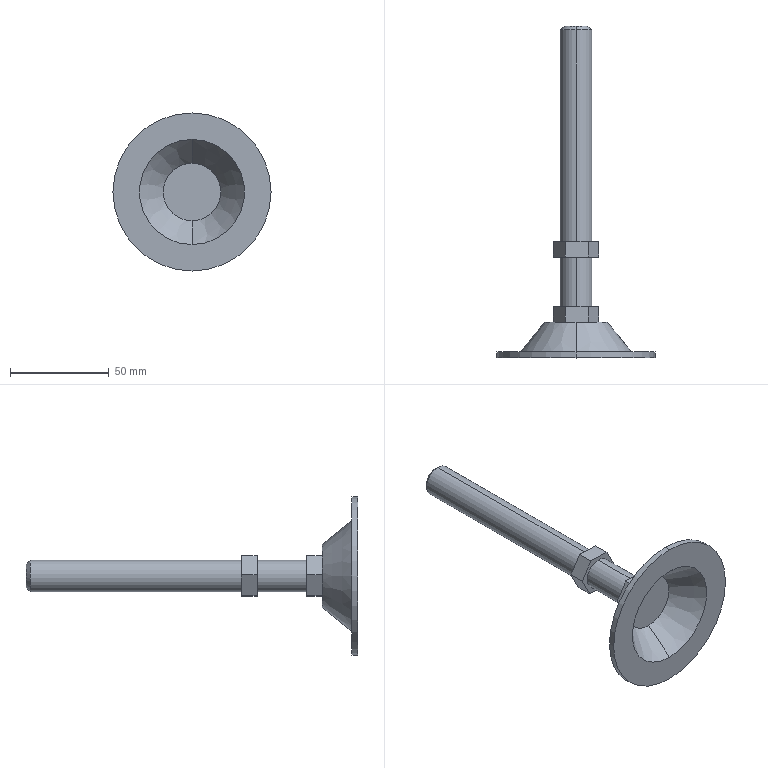Part | SolidWorks | features MBimport 1 | 1 solid | 72 faces | box 80 x 168 x 80 mm | volume 50358 mm3 | plane 46 | cone 12 | spline 8 | cylinder 6 | commonest cylinder face diameters 16 x4 80 x2